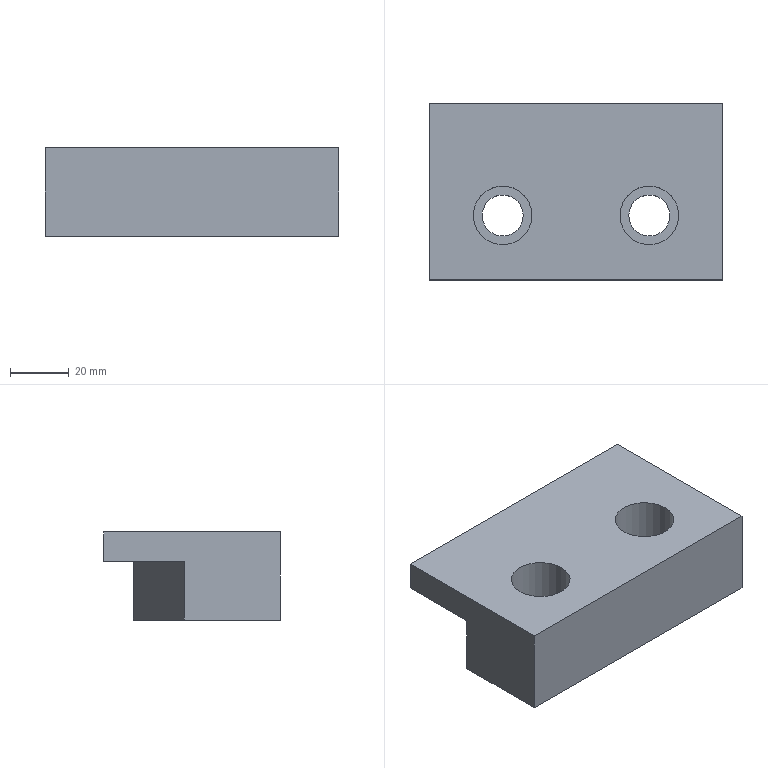Part | NX | features solid 2 | 1 solid | 15 faces | box 100 x 60 x 30 mm | volume 139159 mm3 | plane 11 | cylinder 4 | commonest cylinder face diameters 14 x2 20 x2
STEP:
#1=CARTESIAN_POINT('',(-1267.,-448.,0.));
#2=VERTEX_POINT('',#1);
#3=CARTESIAN_POINT('',(-1260.,-448.,0.));
#4=DIRECTION('',(0.,0.,1.));
#5=DIRECTION('',(-1.,0.,0.));
#6=AXIS2_PLACEMENT_3D('',#3,#4,#5);
#7=CIRCLE('',#6,7.);
#8=EDGE_CURVE('',#2,#2,#7,.T.);
#9=ORIENTED_EDGE('',*,*,#8,.T.);
#10=EDGE_LOOP('',(#9));
#11=FACE_BOUND('',#10,.T.);
#12=CARTESIAN_POINT('',(-1317.,-448.,0.));
#13=VERTEX_POINT('',#12);
#14=CARTESIAN_POINT('',(-1310.,-448.,0.));
#15=DIRECTION('',(0.,0.,1.));
#16=DIRECTION('',(-1.,0.,0.));
#17=AXIS2_PLACEMENT_3D('',#14,#15,#16);
#18=CIRCLE('',#17,7.);
#19=EDGE_CURVE('',#13,#13,#18,.T.);
#20=ORIENTED_EDGE('',*,*,#19,.T.);
#21=EDGE_LOOP('',(#20));
#22=FACE_BOUND('',#21,.T.);
#23=CARTESIAN_POINT('',(-1305.,-420.,0.));
#24=VERTEX_POINT('',#23);
#25=CARTESIAN_POINT('',(-1235.,-420.,0.));
#26=VERTEX_POINT('',#25);
#27=CARTESIAN_POINT('',(-1335.,-420.,0.));
#28=DIRECTION('',(1.,0.,0.));
#29=VECTOR('',#28,1000.);
#30=LINE('',#27,#29);
#31=EDGE_CURVE('',#24,#26,#30,.T.);
#32=ORIENTED_EDGE('',*,*,#31,.T.);
#33=CARTESIAN_POINT('',(-1235.,-470.,0.));
#34=VERTEX_POINT('',#33);
#35=CARTESIAN_POINT('',(-1235.,-470.,0.));
#36=DIRECTION('',(0.,1.,0.));
#37=VECTOR('',#36,1000.);
#38=LINE('',#35,#37);
#39=EDGE_CURVE('',#34,#26,#38,.T.);
#40=ORIENTED_EDGE('',*,*,#39,.F.);
#41=CARTESIAN_POINT('',(-1335.,-470.,0.));
#42=VERTEX_POINT('',#41);
#43=CARTESIAN_POINT('',(-1335.,-470.,0.));
#44=DIRECTION('',(1.,0.,0.));
#45=VECTOR('',#44,1000.);
#46=LINE('',#43,#45);
#47=EDGE_CURVE('',#42,#34,#46,.T.);
#48=ORIENTED_EDGE('',*,*,#47,.F.);
#49=CARTESIAN_POINT('',(-1335.,-437.321,0.));
#50=VERTEX_POINT('',#49);
#51=CARTESIAN_POINT('',(-1335.,-470.,0.));
#52=DIRECTION('',(0.,1.,0.));
#53=VECTOR('',#52,1000.);
#54=LINE('',#51,#53);
#55=EDGE_CURVE('',#42,#50,#54,.T.);
#56=ORIENTED_EDGE('',*,*,#55,.T.);
#57=CARTESIAN_POINT('',(-1391.603,-470.,0.));
#58=DIRECTION('',(0.866,0.5,0.));
#59=VECTOR('',#58,1000.);
#60=LINE('',#57,#59);
#61=EDGE_CURVE('',#50,#24,#60,.T.);
#62=ORIENTED_EDGE('',*,*,#61,.T.);
#63=EDGE_LOOP('',(#32,#40,#48,#56,#62));
#64=FACE_BOUND('',#63,.T.);
#65=CARTESIAN_POINT('',(-1335.,-470.,0.));
#66=DIRECTION('',(0.,0.,-1.));
#67=DIRECTION('',(-1.,0.,0.));
#68=AXIS2_PLACEMENT_3D('',#65,#66,#67);
#69=PLANE('',#68);
#70=ADVANCED_FACE('',(#11,#22,#64),#69,.T.);
#71=CARTESIAN_POINT('',(-1305.,-420.,20.));
#72=VERTEX_POINT('',#71);
#73=CARTESIAN_POINT('',(-1305.,-420.,0.));
#74=DIRECTION('',(0.,0.,1.));
#75=VECTOR('',#74,1000.);
#76=LINE('',#73,#75);
#77=EDGE_CURVE('',#24,#72,#76,.T.);
#78=ORIENTED_EDGE('',*,*,#77,.T.);
#79=CARTESIAN_POINT('',(-1235.,-420.,20.));
#80=VERTEX_POINT('',#79);
#81=CARTESIAN_POINT('',(-1335.,-420.,20.));
#82=DIRECTION('',(1.,0.,0.));
#83=VECTOR('',#82,1000.);
#84=LINE('',#81,#83);
#85=EDGE_CURVE('',#72,#80,#84,.T.);
#86=ORIENTED_EDGE('',*,*,#85,.T.);
#87=CARTESIAN_POINT('',(-1235.,-420.,0.));
#88=DIRECTION('',(0.,0.,1.));
#89=VECTOR('',#88,1000.);
#90=LINE('',#87,#89);
#91=EDGE_CURVE('',#26,#80,#90,.T.);
#92=ORIENTED_EDGE('',*,*,#91,.F.);
#93=ORIENTED_EDGE('',*,*,#31,.F.);
#94=EDGE_LOOP('',(#78,#86,#92,#93));
#95=FACE_BOUND('',#94,.T.);
#96=CARTESIAN_POINT('',(-1335.,-420.,0.));
#97=DIRECTION('',(0.,1.,0.));
#98=DIRECTION('',(1.,0.,0.));
#99=AXIS2_PLACEMENT_3D('',#96,#97,#98);
#100=PLANE('',#99);
#101=ADVANCED_FACE('',(#95),#100,.T.);
#102=CARTESIAN_POINT('',(-1335.,-470.,30.));
#103=VERTEX_POINT('',#102);
#104=CARTESIAN_POINT('',(-1335.,-470.,0.));
#105=DIRECTION('',(0.,0.,-1.));
#106=VECTOR('',#105,1000.);
#107=LINE('',#104,#106);
#108=EDGE_CURVE('',#42,#103,#107,.F.);
#109=ORIENTED_EDGE('',*,*,#108,.F.);
#110=ORIENTED_EDGE('',*,*,#47,.T.);
#111=CARTESIAN_POINT('',(-1235.,-470.,30.));
#112=VERTEX_POINT('',#111);
#113=CARTESIAN_POINT('',(-1235.,-470.,0.));
#114=DIRECTION('',(0.,0.,-1.));
#115=VECTOR('',#114,1000.);
#116=LINE('',#113,#115);
#117=EDGE_CURVE('',#34,#112,#116,.F.);
#118=ORIENTED_EDGE('',*,*,#117,.T.);
#119=CARTESIAN_POINT('',(-1335.,-470.,30.));
#120=DIRECTION('',(-1.,0.,0.));
#121=VECTOR('',#120,1000.);
#122=LINE('',#119,#121);
#123=EDGE_CURVE('',#103,#112,#122,.F.);
#124=ORIENTED_EDGE('',*,*,#123,.F.);
#125=EDGE_LOOP('',(#109,#110,#118,#124));
#126=FACE_BOUND('',#125,.T.);
#127=CARTESIAN_POINT('',(-1335.,-470.,0.));
#128=DIRECTION('',(0.,-1.,0.));
#129=DIRECTION('',(1.,0.,0.));
#130=AXIS2_PLACEMENT_3D('',#127,#128,#129);
#131=PLANE('',#130);
#132=ADVANCED_FACE('',(#126),#131,.T.);
#133=CARTESIAN_POINT('',(-1235.,-410.,20.));
#134=VERTEX_POINT('',#133);
#135=CARTESIAN_POINT('',(-1235.,-410.,20.));
#136=DIRECTION('',(0.,-1.,0.));
#137=VECTOR('',#136,1000.);
#138=LINE('',#135,#137);
#139=EDGE_CURVE('',#134,#80,#138,.T.);
#140=ORIENTED_EDGE('',*,*,#139,.F.);
#141=CARTESIAN_POINT('',(-1235.,-410.,30.));
#142=VERTEX_POINT('',#141);
#143=CARTESIAN_POINT('',(-1235.,-410.,0.));
#144=DIRECTION('',(0.,0.,-1.));
#145=VECTOR('',#144,1000.);
#146=LINE('',#143,#145);
#147=EDGE_CURVE('',#134,#142,#146,.F.);
#148=ORIENTED_EDGE('',*,*,#147,.T.);
#149=CARTESIAN_POINT('',(-1235.,-470.,30.));
#150=DIRECTION('',(0.,-1.,0.));
#151=VECTOR('',#150,1000.);
#152=LINE('',#149,#151);
#153=EDGE_CURVE('',#112,#142,#152,.F.);
#154=ORIENTED_EDGE('',*,*,#153,.F.);
#155=ORIENTED_EDGE('',*,*,#117,.F.);
#156=ORIENTED_EDGE('',*,*,#39,.T.);
#157=ORIENTED_EDGE('',*,*,#91,.T.);
#158=EDGE_LOOP('',(#140,#148,#154,#155,#156,#157));
#159=FACE_BOUND('',#158,.T.);
#160=CARTESIAN_POINT('',(-1235.,-470.,0.));
#161=DIRECTION('',(1.,0.,0.));
#162=DIRECTION('',(0.,1.,0.));
#163=AXIS2_PLACEMENT_3D('',#160,#161,#162);
#164=PLANE('',#163);
#165=ADVANCED_FACE('',(#159),#164,.T.);
#166=CARTESIAN_POINT('',(-1335.,-410.,20.));
#167=VERTEX_POINT('',#166);
#168=CARTESIAN_POINT('',(-1335.,-410.,30.));
#169=VERTEX_POINT('',#168);
#170=CARTESIAN_POINT('',(-1335.,-410.,0.));
#171=DIRECTION('',(0.,0.,-1.));
#172=VECTOR('',#171,1000.);
#173=LINE('',#170,#172);
#174=EDGE_CURVE('',#167,#169,#173,.F.);
#175=ORIENTED_EDGE('',*,*,#174,.T.);
#176=CARTESIAN_POINT('',(-1335.,-410.,30.));
#177=DIRECTION('',(1.,0.,0.));
#178=VECTOR('',#177,1000.);
#179=LINE('',#176,#178);
#180=EDGE_CURVE('',#169,#142,#179,.T.);
#181=ORIENTED_EDGE('',*,*,#180,.T.);
#182=ORIENTED_EDGE('',*,*,#147,.F.);
#183=CARTESIAN_POINT('',(-1335.,-410.,20.));
#184=DIRECTION('',(1.,0.,0.));
#185=VECTOR('',#184,1000.);
#186=LINE('',#183,#185);
#187=EDGE_CURVE('',#167,#134,#186,.T.);
#188=ORIENTED_EDGE('',*,*,#187,.F.);
#189=EDGE_LOOP('',(#175,#181,#182,#188));
#190=FACE_BOUND('',#189,.T.);
#191=CARTESIAN_POINT('',(-1335.,-410.,0.));
#192=DIRECTION('',(0.,-1.,0.));
#193=DIRECTION('',(1.,0.,0.));
#194=AXIS2_PLACEMENT_3D('',#191,#192,#193);
#195=PLANE('',#194);
#196=ADVANCED_FACE('',(#190),#195,.F.);
#197=CARTESIAN_POINT('',(-1335.,-437.321,20.));
#198=VERTEX_POINT('',#197);
#199=CARTESIAN_POINT('',(-1335.,-437.321,0.));
#200=DIRECTION('',(0.,0.,-1.));
#201=VECTOR('',#200,1000.);
#202=LINE('',#199,#201);
#203=EDGE_CURVE('',#198,#50,#202,.T.);
#204=ORIENTED_EDGE('',*,*,#203,.T.);
#205=ORIENTED_EDGE('',*,*,#55,.F.);
#206=ORIENTED_EDGE('',*,*,#108,.T.);
#207=CARTESIAN_POINT('',(-1335.,-470.,30.));
#208=DIRECTION('',(0.,1.,0.));
#209=VECTOR('',#208,1000.);
#210=LINE('',#207,#209);
#211=EDGE_CURVE('',#103,#169,#210,.T.);
#212=ORIENTED_EDGE('',*,*,#211,.T.);
#213=ORIENTED_EDGE('',*,*,#174,.F.);
#214=CARTESIAN_POINT('',(-1335.,-410.,20.));
#215=DIRECTION('',(0.,-1.,0.));
#216=VECTOR('',#215,1000.);
#217=LINE('',#214,#216);
#218=EDGE_CURVE('',#167,#198,#217,.T.);
#219=ORIENTED_EDGE('',*,*,#218,.T.);
#220=EDGE_LOOP('',(#204,#205,#206,#212,#213,#219));
#221=FACE_BOUND('',#220,.T.);
#222=CARTESIAN_POINT('',(-1335.,-470.,0.));
#223=DIRECTION('',(1.,0.,0.));
#224=DIRECTION('',(0.,1.,0.));
#225=AXIS2_PLACEMENT_3D('',#222,#223,#224);
#226=PLANE('',#225);
#227=ADVANCED_FACE('',(#221),#226,.F.);
#228=CARTESIAN_POINT('',(-1270.,-448.,30.));
#229=VERTEX_POINT('',#228);
#230=CARTESIAN_POINT('',(-1260.,-448.,30.));
#231=DIRECTION('',(0.,0.,1.));
#232=DIRECTION('',(-1.,0.,0.));
#233=AXIS2_PLACEMENT_3D('',#230,#231,#232);
#234=CIRCLE('',#233,10.);
#235=EDGE_CURVE('',#229,#229,#234,.T.);
#236=ORIENTED_EDGE('',*,*,#235,.F.);
#237=EDGE_LOOP('',(#236));
#238=FACE_BOUND('',#237,.T.);
#239=CARTESIAN_POINT('',(-1320.,-448.,30.));
#240=VERTEX_POINT('',#239);
#241=CARTESIAN_POINT('',(-1310.,-448.,30.));
#242=DIRECTION('',(0.,0.,1.));
#243=DIRECTION('',(-1.,0.,0.));
#244=AXIS2_PLACEMENT_3D('',#241,#242,#243);
#245=CIRCLE('',#244,10.);
#246=EDGE_CURVE('',#240,#240,#245,.T.);
#247=ORIENTED_EDGE('',*,*,#246,.F.);
#248=EDGE_LOOP('',(#247));
#249=FACE_BOUND('',#248,.T.);
#250=ORIENTED_EDGE('',*,*,#180,.F.);
#251=ORIENTED_EDGE('',*,*,#211,.F.);
#252=ORIENTED_EDGE('',*,*,#123,.T.);
#253=ORIENTED_EDGE('',*,*,#153,.T.);
#254=EDGE_LOOP('',(#250,#251,#252,#253));
#255=FACE_BOUND('',#254,.T.);
#256=CARTESIAN_POINT('',(-1335.,-470.,30.));
#257=DIRECTION('',(0.,0.,-1.));
#258=DIRECTION('',(-1.,0.,0.));
#259=AXIS2_PLACEMENT_3D('',#256,#257,#258);
#260=PLANE('',#259);
#261=ADVANCED_FACE('',(#238,#249,#255),#260,.F.);
#262=ORIENTED_EDGE('',*,*,#139,.T.);
#263=ORIENTED_EDGE('',*,*,#85,.F.);
#264=CARTESIAN_POINT('',(-1391.603,-470.,20.));
#265=DIRECTION('',(0.866,0.5,0.));
#266=VECTOR('',#265,1000.);
#267=LINE('',#264,#266);
#268=EDGE_CURVE('',#198,#72,#267,.T.);
#269=ORIENTED_EDGE('',*,*,#268,.F.);
#270=ORIENTED_EDGE('',*,*,#218,.F.);
#271=ORIENTED_EDGE('',*,*,#187,.T.);
#272=EDGE_LOOP('',(#262,#263,#269,#270,#271));
#273=FACE_BOUND('',#272,.T.);
#274=CARTESIAN_POINT('',(-1335.,-410.,20.));
#275=DIRECTION('',(0.,0.,1.));
#276=DIRECTION('',(1.,0.,0.));
#277=AXIS2_PLACEMENT_3D('',#274,#275,#276);
#278=PLANE('',#277);
#279=ADVANCED_FACE('',(#273),#278,.F.);
#280=ORIENTED_EDGE('',*,*,#203,.F.);
#281=ORIENTED_EDGE('',*,*,#268,.T.);
#282=ORIENTED_EDGE('',*,*,#77,.F.);
#283=ORIENTED_EDGE('',*,*,#61,.F.);
#284=EDGE_LOOP('',(#280,#281,#282,#283));
#285=FACE_BOUND('',#284,.T.);
#286=CARTESIAN_POINT('',(-1391.603,-470.,0.));
#287=DIRECTION('',(-0.5,0.866,0.));
#288=DIRECTION('',(0.866,0.5,0.));
#289=AXIS2_PLACEMENT_3D('',#286,#287,#288);
#290=PLANE('',#289);
#291=ADVANCED_FACE('',(#285),#290,.T.);
#292=ORIENTED_EDGE('',*,*,#19,.F.);
#293=EDGE_LOOP('',(#292));
#294=FACE_BOUND('',#293,.T.);
#295=CARTESIAN_POINT('',(-1317.,-448.,10.));
#296=VERTEX_POINT('',#295);
#297=CARTESIAN_POINT('',(-1310.,-448.,10.));
#298=DIRECTION('',(0.,0.,1.));
#299=DIRECTION('',(-1.,0.,0.));
#300=AXIS2_PLACEMENT_3D('',#297,#298,#299);
#301=CIRCLE('',#300,7.);
#302=EDGE_CURVE('',#296,#296,#301,.T.);
#303=ORIENTED_EDGE('',*,*,#302,.T.);
#304=EDGE_LOOP('',(#303));
#305=FACE_BOUND('',#304,.T.);
#306=CARTESIAN_POINT('',(-1310.,-448.,-20.));
#307=DIRECTION('',(0.,0.,-1.));
#308=DIRECTION('',(-1.,0.,0.));
#309=AXIS2_PLACEMENT_3D('',#306,#307,#308);
#310=CYLINDRICAL_SURFACE('',#309,7.);
#311=ADVANCED_FACE('',(#294,#305),#310,.F.);
#312=ORIENTED_EDGE('',*,*,#302,.F.);
#313=EDGE_LOOP('',(#312));
#314=FACE_BOUND('',#313,.T.);
#315=CARTESIAN_POINT('',(-1320.,-448.,10.));
#316=VERTEX_POINT('',#315);
#317=CARTESIAN_POINT('',(-1310.,-448.,10.));
#318=DIRECTION('',(0.,0.,1.));
#319=DIRECTION('',(-1.,0.,0.));
#320=AXIS2_PLACEMENT_3D('',#317,#318,#319);
#321=CIRCLE('',#320,10.);
#322=EDGE_CURVE('',#316,#316,#321,.T.);
#323=ORIENTED_EDGE('',*,*,#322,.T.);
#324=EDGE_LOOP('',(#323));
#325=FACE_BOUND('',#324,.T.);
#326=CARTESIAN_POINT('',(-1310.,-448.,10.));
#327=DIRECTION('',(0.,0.,-1.));
#328=DIRECTION('',(-1.,0.,0.));
#329=AXIS2_PLACEMENT_3D('',#326,#327,#328);
#330=PLANE('',#329);
#331=ADVANCED_FACE('',(#314,#325),#330,.F.);
#332=ORIENTED_EDGE('',*,*,#322,.F.);
#333=EDGE_LOOP('',(#332));
#334=FACE_BOUND('',#333,.T.);
#335=ORIENTED_EDGE('',*,*,#246,.T.);
#336=EDGE_LOOP('',(#335));
#337=FACE_BOUND('',#336,.T.);
#338=CARTESIAN_POINT('',(-1310.,-448.,30.));
#339=DIRECTION('',(0.,0.,-1.));
#340=DIRECTION('',(-1.,0.,0.));
#341=AXIS2_PLACEMENT_3D('',#338,#339,#340);
#342=CYLINDRICAL_SURFACE('',#341,10.);
#343=ADVANCED_FACE('',(#334,#337),#342,.F.);
#344=ORIENTED_EDGE('',*,*,#8,.F.);
#345=EDGE_LOOP('',(#344));
#346=FACE_BOUND('',#345,.T.);
#347=CARTESIAN_POINT('',(-1267.,-448.,10.));
#348=VERTEX_POINT('',#347);
#349=CARTESIAN_POINT('',(-1260.,-448.,10.));
#350=DIRECTION('',(0.,0.,1.));
#351=DIRECTION('',(-1.,0.,0.));
#352=AXIS2_PLACEMENT_3D('',#349,#350,#351);
#353=CIRCLE('',#352,7.);
#354=EDGE_CURVE('',#348,#348,#353,.T.);
#355=ORIENTED_EDGE('',*,*,#354,.T.);
#356=EDGE_LOOP('',(#355));
#357=FACE_BOUND('',#356,.T.);
#358=CARTESIAN_POINT('',(-1260.,-448.,-20.));
#359=DIRECTION('',(0.,0.,-1.));
#360=DIRECTION('',(-1.,0.,0.));
#361=AXIS2_PLACEMENT_3D('',#358,#359,#360);
#362=CYLINDRICAL_SURFACE('',#361,7.);
#363=ADVANCED_FACE('',(#346,#357),#362,.F.);
#364=ORIENTED_EDGE('',*,*,#354,.F.);
#365=EDGE_LOOP('',(#364));
#366=FACE_BOUND('',#365,.T.);
#367=CARTESIAN_POINT('',(-1270.,-448.,10.));
#368=VERTEX_POINT('',#367);
#369=CARTESIAN_POINT('',(-1260.,-448.,10.));
#370=DIRECTION('',(0.,0.,1.));
#371=DIRECTION('',(-1.,0.,0.));
#372=AXIS2_PLACEMENT_3D('',#369,#370,#371);
#373=CIRCLE('',#372,10.);
#374=EDGE_CURVE('',#368,#368,#373,.T.);
#375=ORIENTED_EDGE('',*,*,#374,.T.);
#376=EDGE_LOOP('',(#375));
#377=FACE_BOUND('',#376,.T.);
#378=CARTESIAN_POINT('',(-1260.,-448.,10.));
#379=DIRECTION('',(0.,0.,-1.));
#380=DIRECTION('',(-1.,0.,0.));
#381=AXIS2_PLACEMENT_3D('',#378,#379,#380);
#382=PLANE('',#381);
#383=ADVANCED_FACE('',(#366,#377),#382,.F.);
#384=ORIENTED_EDGE('',*,*,#374,.F.);
#385=EDGE_LOOP('',(#384));
#386=FACE_BOUND('',#385,.T.);
#387=ORIENTED_EDGE('',*,*,#235,.T.);
#388=EDGE_LOOP('',(#387));
#389=FACE_BOUND('',#388,.T.);
#390=CARTESIAN_POINT('',(-1260.,-448.,30.));
#391=DIRECTION('',(0.,0.,-1.));
#392=DIRECTION('',(-1.,0.,0.));
#393=AXIS2_PLACEMENT_3D('',#390,#391,#392);
#394=CYLINDRICAL_SURFACE('',#393,10.);
#395=ADVANCED_FACE('',(#386,#389),#394,.F.);
#396=CLOSED_SHELL('',(#70,#101,#132,#165,#196,#227,#261,#279,#291,#311,#331,#343,#363,#383,#395));
#397=MANIFOLD_SOLID_BREP('',#396);
#398=(LENGTH_UNIT()NAMED_UNIT(*)SI_UNIT(.MILLI.,.METRE.));
#399=UNCERTAINTY_MEASURE_WITH_UNIT(LENGTH_MEASURE(0.00001),#398,'','');
#400=(NAMED_UNIT(*)PLANE_ANGLE_UNIT()SI_UNIT($,.RADIAN.));
#401=(NAMED_UNIT(*)SI_UNIT($,.STERADIAN.)SOLID_ANGLE_UNIT());
#402=(GEOMETRIC_REPRESENTATION_CONTEXT(3)GLOBAL_UNCERTAINTY_ASSIGNED_CONTEXT((#399))GLOBAL_UNIT_ASSIGNED_CONTEXT((#398,#400,#401))REPRESENTATION_CONTEXT('',''));
#403=ADVANCED_BREP_SHAPE_REPRESENTATION('',(#397),#402);